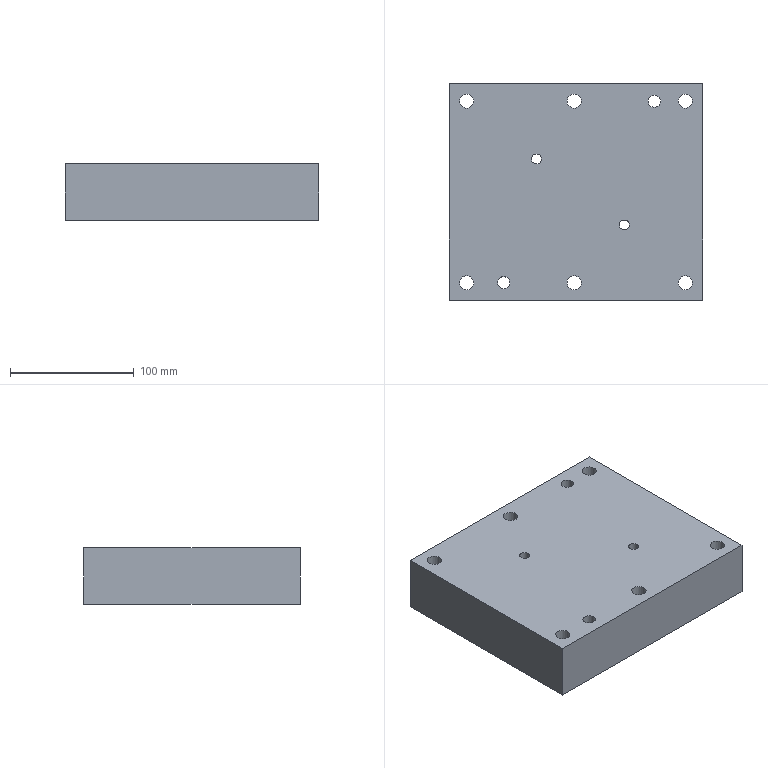Part | NX | features solid 2 | 1 solid | 50 faces | box 205 x 175 x 46 mm | volume 1591427 mm3 | cylinder 24 | plane 14 | cone 12 | commonest cylinder face diameters 6.8 x6 11.507 x6 18.008 x6 8 x2 10 x2 12.505 x2
STEP:
#1=CARTESIAN_POINT('',(-87.57,-13.004,130.));
#2=VERTEX_POINT('',#1);
#3=CARTESIAN_POINT('',(-90.97,-13.004,130.));
#4=DIRECTION('',(0.,0.,1.));
#5=DIRECTION('',(1.,0.,0.));
#6=AXIS2_PLACEMENT_3D('',#3,#4,#5);
#7=CIRCLE('',#6,3.4);
#8=EDGE_CURVE('',#2,#2,#7,.F.);
#9=ORIENTED_EDGE('',*,*,#8,.T.);
#10=EDGE_LOOP('',(#9));
#11=FACE_BOUND('',#10,.T.);
#12=CARTESIAN_POINT('',(-90.97,-13.004,132.043));
#13=VERTEX_POINT('',#12);
#14=VERTEX_LOOP('',#13);
#15=FACE_BOUND('',#14,.T.);
#16=CARTESIAN_POINT('',(-90.97,-13.004,130.));
#17=DIRECTION('',(0.,0.,-1.));
#18=DIRECTION('',(-1.,0.,0.));
#19=AXIS2_PLACEMENT_3D('',#16,#17,#18);
#20=CONICAL_SURFACE('',#19,3.4,1.03);
#21=ADVANCED_FACE('',(#11,#15),#20,.F.);
#22=CARTESIAN_POINT('',(-94.37,-13.004,105.599));
#23=VERTEX_POINT('',#22);
#24=CARTESIAN_POINT('',(-90.97,-13.004,105.599));
#25=DIRECTION('',(0.,0.,-1.));
#26=DIRECTION('',(-1.,0.,0.));
#27=AXIS2_PLACEMENT_3D('',#24,#25,#26);
#28=CIRCLE('',#27,3.4);
#29=EDGE_CURVE('',#23,#23,#28,.T.);
#30=ORIENTED_EDGE('',*,*,#29,.T.);
#31=EDGE_LOOP('',(#30));
#32=FACE_BOUND('',#31,.T.);
#33=ORIENTED_EDGE('',*,*,#8,.F.);
#34=EDGE_LOOP('',(#33));
#35=FACE_BOUND('',#34,.T.);
#36=CARTESIAN_POINT('',(-90.97,-13.004,105.));
#37=DIRECTION('',(0.,0.,1.));
#38=DIRECTION('',(1.,0.,0.));
#39=AXIS2_PLACEMENT_3D('',#36,#37,#38);
#40=CYLINDRICAL_SURFACE('',#39,3.4);
#41=ADVANCED_FACE('',(#32,#35),#40,.F.);
#42=CARTESIAN_POINT('',(-87.101,-13.004,105.13));
#43=VERTEX_POINT('',#42);
#44=CARTESIAN_POINT('',(-90.97,-13.004,105.13));
#45=DIRECTION('',(0.,0.,1.));
#46=DIRECTION('',(1.,0.,0.));
#47=AXIS2_PLACEMENT_3D('',#44,#45,#46);
#48=CIRCLE('',#47,3.869);
#49=EDGE_CURVE('',#43,#43,#48,.F.);
#50=ORIENTED_EDGE('',*,*,#49,.T.);
#51=EDGE_LOOP('',(#50));
#52=FACE_BOUND('',#51,.T.);
#53=ORIENTED_EDGE('',*,*,#29,.F.);
#54=EDGE_LOOP('',(#53));
#55=FACE_BOUND('',#54,.T.);
#56=CARTESIAN_POINT('',(-90.97,-13.004,105.599));
#57=DIRECTION('',(0.,0.,-1.));
#58=DIRECTION('',(-1.,0.,0.));
#59=AXIS2_PLACEMENT_3D('',#56,#57,#58);
#60=CONICAL_SURFACE('',#59,3.4,0.7854);
#61=ADVANCED_FACE('',(#52,#55),#60,.F.);
#62=CARTESIAN_POINT('',(-252.523,47.776,105.13));
#63=VERTEX_POINT('',#62);
#64=CARTESIAN_POINT('',(-47.523,47.776,105.13));
#65=VERTEX_POINT('',#64);
#66=CARTESIAN_POINT('',(-150.023,47.776,105.13));
#67=DIRECTION('',(1.,0.,0.));
#68=VECTOR('',#67,1000.);
#69=LINE('',#66,#68);
#70=EDGE_CURVE('',#63,#65,#69,.T.);
#71=ORIENTED_EDGE('',*,*,#70,.T.);
#72=CARTESIAN_POINT('',(-47.523,-127.224,105.13));
#73=VERTEX_POINT('',#72);
#74=CARTESIAN_POINT('',(-47.523,-39.724,105.13));
#75=DIRECTION('',(0.,-1.,0.));
#76=VECTOR('',#75,1000.);
#77=LINE('',#74,#76);
#78=EDGE_CURVE('',#73,#65,#77,.F.);
#79=ORIENTED_EDGE('',*,*,#78,.F.);
#80=CARTESIAN_POINT('',(-252.523,-127.224,105.13));
#81=VERTEX_POINT('',#80);
#82=CARTESIAN_POINT('',(-150.023,-127.224,105.13));
#83=DIRECTION('',(-1.,0.,0.));
#84=VECTOR('',#83,1000.);
#85=LINE('',#82,#84);
#86=EDGE_CURVE('',#81,#73,#85,.F.);
#87=ORIENTED_EDGE('',*,*,#86,.F.);
#88=CARTESIAN_POINT('',(-252.523,-39.724,105.13));
#89=DIRECTION('',(0.,1.,0.));
#90=VECTOR('',#89,1000.);
#91=LINE('',#88,#90);
#92=EDGE_CURVE('',#63,#81,#91,.F.);
#93=ORIENTED_EDGE('',*,*,#92,.F.);
#94=EDGE_LOOP('',(#71,#79,#87,#93));
#95=FACE_BOUND('',#94,.T.);
#96=CARTESIAN_POINT('',(-229.519,-113.224,105.13));
#97=VERTEX_POINT('',#96);
#98=CARTESIAN_POINT('',(-238.523,-113.224,105.13));
#99=DIRECTION('',(0.,0.,1.));
#100=DIRECTION('',(1.,0.,0.));
#101=AXIS2_PLACEMENT_3D('',#98,#99,#100);
#102=CIRCLE('',#101,9.004);
#103=EDGE_CURVE('',#97,#97,#102,.T.);
#104=ORIENTED_EDGE('',*,*,#103,.T.);
#105=EDGE_LOOP('',(#104));
#106=FACE_BOUND('',#105,.T.);
#107=CARTESIAN_POINT('',(-52.519,-113.224,105.13));
#108=VERTEX_POINT('',#107);
#109=CARTESIAN_POINT('',(-61.523,-113.224,105.13));
#110=DIRECTION('',(0.,0.,1.));
#111=DIRECTION('',(1.,0.,0.));
#112=AXIS2_PLACEMENT_3D('',#109,#110,#111);
#113=CIRCLE('',#112,9.004);
#114=EDGE_CURVE('',#108,#108,#113,.F.);
#115=ORIENTED_EDGE('',*,*,#114,.F.);
#116=EDGE_LOOP('',(#115));
#117=FACE_BOUND('',#116,.T.);
#118=CARTESIAN_POINT('',(-202.271,-113.224,105.13));
#119=VERTEX_POINT('',#118);
#120=CARTESIAN_POINT('',(-208.523,-113.224,105.13));
#121=DIRECTION('',(0.,0.,1.));
#122=DIRECTION('',(1.,0.,0.));
#123=AXIS2_PLACEMENT_3D('',#120,#121,#122);
#124=CIRCLE('',#123,6.253);
#125=EDGE_CURVE('',#119,#119,#124,.T.);
#126=ORIENTED_EDGE('',*,*,#125,.T.);
#127=EDGE_LOOP('',(#126));
#128=FACE_BOUND('',#127,.T.);
#129=CARTESIAN_POINT('',(-142.519,33.776,105.13));
#130=VERTEX_POINT('',#129);
#131=CARTESIAN_POINT('',(-151.523,33.776,105.13));
#132=DIRECTION('',(0.,0.,1.));
#133=DIRECTION('',(1.,0.,0.));
#134=AXIS2_PLACEMENT_3D('',#131,#132,#133);
#135=CIRCLE('',#134,9.004);
#136=EDGE_CURVE('',#130,#130,#135,.F.);
#137=ORIENTED_EDGE('',*,*,#136,.F.);
#138=EDGE_LOOP('',(#137));
#139=FACE_BOUND('',#138,.T.);
#140=ORIENTED_EDGE('',*,*,#49,.F.);
#141=EDGE_LOOP('',(#140));
#142=FACE_BOUND('',#141,.T.);
#143=CARTESIAN_POINT('',(-146.154,-13.004,105.13));
#144=VERTEX_POINT('',#143);
#145=CARTESIAN_POINT('',(-150.023,-13.004,105.13));
#146=DIRECTION('',(0.,0.,1.));
#147=DIRECTION('',(1.,0.,0.));
#148=AXIS2_PLACEMENT_3D('',#145,#146,#147);
#149=CIRCLE('',#148,3.869);
#150=EDGE_CURVE('',#144,#144,#149,.F.);
#151=ORIENTED_EDGE('',*,*,#150,.F.);
#152=EDGE_LOOP('',(#151));
#153=FACE_BOUND('',#152,.T.);
#154=CARTESIAN_POINT('',(-203.207,-13.004,105.13));
#155=VERTEX_POINT('',#154);
#156=CARTESIAN_POINT('',(-207.076,-13.004,105.13));
#157=DIRECTION('',(0.,0.,1.));
#158=DIRECTION('',(1.,0.,0.));
#159=AXIS2_PLACEMENT_3D('',#156,#157,#158);
#160=CIRCLE('',#159,3.869);
#161=EDGE_CURVE('',#155,#155,#160,.T.);
#162=ORIENTED_EDGE('',*,*,#161,.T.);
#163=EDGE_LOOP('',(#162));
#164=FACE_BOUND('',#163,.T.);
#165=CARTESIAN_POINT('',(-203.207,-66.444,105.13));
#166=VERTEX_POINT('',#165);
#167=CARTESIAN_POINT('',(-207.076,-66.444,105.13));
#168=DIRECTION('',(0.,0.,1.));
#169=DIRECTION('',(1.,0.,0.));
#170=AXIS2_PLACEMENT_3D('',#167,#168,#169);
#171=CIRCLE('',#170,3.869);
#172=EDGE_CURVE('',#166,#166,#171,.T.);
#173=ORIENTED_EDGE('',*,*,#172,.T.);
#174=EDGE_LOOP('',(#173));
#175=FACE_BOUND('',#174,.T.);
#176=CARTESIAN_POINT('',(-146.154,-66.444,105.13));
#177=VERTEX_POINT('',#176);
#178=CARTESIAN_POINT('',(-150.023,-66.444,105.13));
#179=DIRECTION('',(0.,0.,1.));
#180=DIRECTION('',(1.,0.,0.));
#181=AXIS2_PLACEMENT_3D('',#178,#179,#180);
#182=CIRCLE('',#181,3.869);
#183=EDGE_CURVE('',#177,#177,#182,.F.);
#184=ORIENTED_EDGE('',*,*,#183,.F.);
#185=EDGE_LOOP('',(#184));
#186=FACE_BOUND('',#185,.T.);
#187=CARTESIAN_POINT('',(-87.101,-66.444,105.13));
#188=VERTEX_POINT('',#187);
#189=CARTESIAN_POINT('',(-90.97,-66.444,105.13));
#190=DIRECTION('',(0.,0.,1.));
#191=DIRECTION('',(1.,0.,0.));
#192=AXIS2_PLACEMENT_3D('',#189,#190,#191);
#193=CIRCLE('',#192,3.869);
#194=EDGE_CURVE('',#188,#188,#193,.F.);
#195=ORIENTED_EDGE('',*,*,#194,.F.);
#196=EDGE_LOOP('',(#195));
#197=FACE_BOUND('',#196,.T.);
#198=CARTESIAN_POINT('',(-111.38,-62.465,105.13));
#199=VERTEX_POINT('',#198);
#200=CARTESIAN_POINT('',(-110.97,-66.444,105.13));
#201=DIRECTION('',(0.,0.,1.));
#202=DIRECTION('',(-0.1024,0.9947,0.));
#203=AXIS2_PLACEMENT_3D('',#200,#201,#202);
#204=ELLIPSE('',#203,4.,4.);
#205=EDGE_CURVE('',#199,#199,#204,.T.);
#206=ORIENTED_EDGE('',*,*,#205,.T.);
#207=EDGE_LOOP('',(#206));
#208=FACE_BOUND('',#207,.T.);
#209=CARTESIAN_POINT('',(-182.486,-9.025,105.13));
#210=VERTEX_POINT('',#209);
#211=CARTESIAN_POINT('',(-182.076,-13.004,105.13));
#212=DIRECTION('',(0.,0.,1.));
#213=DIRECTION('',(-0.1024,0.9947,0.));
#214=AXIS2_PLACEMENT_3D('',#211,#212,#213);
#215=ELLIPSE('',#214,4.,4.);
#216=EDGE_CURVE('',#210,#210,#215,.T.);
#217=ORIENTED_EDGE('',*,*,#216,.T.);
#218=EDGE_LOOP('',(#217));
#219=FACE_BOUND('',#218,.T.);
#220=CARTESIAN_POINT('',(-142.519,-113.224,105.13));
#221=VERTEX_POINT('',#220);
#222=CARTESIAN_POINT('',(-151.523,-113.224,105.13));
#223=DIRECTION('',(0.,0.,1.));
#224=DIRECTION('',(1.,0.,0.));
#225=AXIS2_PLACEMENT_3D('',#222,#223,#224);
#226=CIRCLE('',#225,9.004);
#227=EDGE_CURVE('',#221,#221,#226,.F.);
#228=ORIENTED_EDGE('',*,*,#227,.F.);
#229=EDGE_LOOP('',(#228));
#230=FACE_BOUND('',#229,.T.);
#231=CARTESIAN_POINT('',(-80.271,33.776,105.13));
#232=VERTEX_POINT('',#231);
#233=CARTESIAN_POINT('',(-86.523,33.776,105.13));
#234=DIRECTION('',(0.,0.,1.));
#235=DIRECTION('',(1.,0.,0.));
#236=AXIS2_PLACEMENT_3D('',#233,#234,#235);
#237=CIRCLE('',#236,6.253);
#238=EDGE_CURVE('',#232,#232,#237,.T.);
#239=ORIENTED_EDGE('',*,*,#238,.T.);
#240=EDGE_LOOP('',(#239));
#241=FACE_BOUND('',#240,.T.);
#242=CARTESIAN_POINT('',(-229.519,33.776,105.13));
#243=VERTEX_POINT('',#242);
#244=CARTESIAN_POINT('',(-238.523,33.776,105.13));
#245=DIRECTION('',(0.,0.,1.));
#246=DIRECTION('',(1.,0.,0.));
#247=AXIS2_PLACEMENT_3D('',#244,#245,#246);
#248=CIRCLE('',#247,9.004);
#249=EDGE_CURVE('',#243,#243,#248,.T.);
#250=ORIENTED_EDGE('',*,*,#249,.T.);
#251=EDGE_LOOP('',(#250));
#252=FACE_BOUND('',#251,.T.);
#253=CARTESIAN_POINT('',(-52.519,33.776,105.13));
#254=VERTEX_POINT('',#253);
#255=CARTESIAN_POINT('',(-61.523,33.776,105.13));
#256=DIRECTION('',(0.,0.,1.));
#257=DIRECTION('',(1.,0.,0.));
#258=AXIS2_PLACEMENT_3D('',#255,#256,#257);
#259=CIRCLE('',#258,9.004);
#260=EDGE_CURVE('',#254,#254,#259,.F.);
#261=ORIENTED_EDGE('',*,*,#260,.F.);
#262=EDGE_LOOP('',(#261));
#263=FACE_BOUND('',#262,.T.);
#264=CARTESIAN_POINT('',(-150.023,-39.724,105.13));
#265=DIRECTION('',(0.,0.,1.));
#266=DIRECTION('',(1.,0.,0.));
#267=AXIS2_PLACEMENT_3D('',#264,#265,#266);
#268=PLANE('',#267);
#269=ADVANCED_FACE('',(#95,#106,#117,#128,#139,#142,#153,#164,#175,#186,#197,#208,#219,#230,#241,#252,#263),#268,.F.);
#270=CARTESIAN_POINT('',(-87.57,-66.444,129.999));
#271=VERTEX_POINT('',#270);
#272=CARTESIAN_POINT('',(-90.97,-66.444,129.999));
#273=DIRECTION('',(0.,0.,1.));
#274=DIRECTION('',(1.,0.,0.));
#275=AXIS2_PLACEMENT_3D('',#272,#273,#274);
#276=CIRCLE('',#275,3.4);
#277=EDGE_CURVE('',#271,#271,#276,.F.);
#278=ORIENTED_EDGE('',*,*,#277,.T.);
#279=EDGE_LOOP('',(#278));
#280=FACE_BOUND('',#279,.T.);
#281=CARTESIAN_POINT('',(-90.97,-66.444,132.042));
#282=VERTEX_POINT('',#281);
#283=VERTEX_LOOP('',#282);
#284=FACE_BOUND('',#283,.T.);
#285=CARTESIAN_POINT('',(-90.97,-66.444,129.999));
#286=DIRECTION('',(0.,0.,-1.));
#287=DIRECTION('',(-1.,0.,0.));
#288=AXIS2_PLACEMENT_3D('',#285,#286,#287);
#289=CONICAL_SURFACE('',#288,3.4,1.03);
#290=ADVANCED_FACE('',(#280,#284),#289,.F.);
#291=CARTESIAN_POINT('',(-94.37,-66.444,105.599));
#292=VERTEX_POINT('',#291);
#293=CARTESIAN_POINT('',(-90.97,-66.444,105.599));
#294=DIRECTION('',(0.,0.,-1.));
#295=DIRECTION('',(-1.,0.,0.));
#296=AXIS2_PLACEMENT_3D('',#293,#294,#295);
#297=CIRCLE('',#296,3.4);
#298=EDGE_CURVE('',#292,#292,#297,.T.);
#299=ORIENTED_EDGE('',*,*,#298,.T.);
#300=EDGE_LOOP('',(#299));
#301=FACE_BOUND('',#300,.T.);
#302=ORIENTED_EDGE('',*,*,#277,.F.);
#303=EDGE_LOOP('',(#302));
#304=FACE_BOUND('',#303,.T.);
#305=CARTESIAN_POINT('',(-90.97,-66.444,104.999));
#306=DIRECTION('',(0.,0.,1.));
#307=DIRECTION('',(1.,0.,0.));
#308=AXIS2_PLACEMENT_3D('',#305,#306,#307);
#309=CYLINDRICAL_SURFACE('',#308,3.4);
#310=ADVANCED_FACE('',(#301,#304),#309,.F.);
#311=ORIENTED_EDGE('',*,*,#194,.T.);
#312=EDGE_LOOP('',(#311));
#313=FACE_BOUND('',#312,.T.);
#314=ORIENTED_EDGE('',*,*,#298,.F.);
#315=EDGE_LOOP('',(#314));
#316=FACE_BOUND('',#315,.T.);
#317=CARTESIAN_POINT('',(-90.97,-66.444,105.599));
#318=DIRECTION('',(0.,0.,-1.));
#319=DIRECTION('',(-1.,0.,0.));
#320=AXIS2_PLACEMENT_3D('',#317,#318,#319);
#321=CONICAL_SURFACE('',#320,3.4,0.7854);
#322=ADVANCED_FACE('',(#313,#316),#321,.F.);
#323=CARTESIAN_POINT('',(-146.623,-66.444,130.));
#324=VERTEX_POINT('',#323);
#325=CARTESIAN_POINT('',(-150.023,-66.444,130.));
#326=DIRECTION('',(0.,0.,1.));
#327=DIRECTION('',(1.,0.,0.));
#328=AXIS2_PLACEMENT_3D('',#325,#326,#327);
#329=CIRCLE('',#328,3.4);
#330=EDGE_CURVE('',#324,#324,#329,.F.);
#331=ORIENTED_EDGE('',*,*,#330,.T.);
#332=EDGE_LOOP('',(#331));
#333=FACE_BOUND('',#332,.T.);
#334=CARTESIAN_POINT('',(-150.023,-66.444,132.042));
#335=VERTEX_POINT('',#334);
#336=VERTEX_LOOP('',#335);
#337=FACE_BOUND('',#336,.T.);
#338=CARTESIAN_POINT('',(-150.023,-66.444,130.));
#339=DIRECTION('',(0.,0.,-1.));
#340=DIRECTION('',(-1.,0.,0.));
#341=AXIS2_PLACEMENT_3D('',#338,#339,#340);
#342=CONICAL_SURFACE('',#341,3.4,1.03);
#343=ADVANCED_FACE('',(#333,#337),#342,.F.);
#344=CARTESIAN_POINT('',(-153.423,-66.444,105.599));
#345=VERTEX_POINT('',#344);
#346=CARTESIAN_POINT('',(-150.023,-66.444,105.599));
#347=DIRECTION('',(0.,0.,-1.));
#348=DIRECTION('',(-1.,0.,0.));
#349=AXIS2_PLACEMENT_3D('',#346,#347,#348);
#350=CIRCLE('',#349,3.4);
#351=EDGE_CURVE('',#345,#345,#350,.T.);
#352=ORIENTED_EDGE('',*,*,#351,.T.);
#353=EDGE_LOOP('',(#352));
#354=FACE_BOUND('',#353,.T.);
#355=ORIENTED_EDGE('',*,*,#330,.F.);
#356=EDGE_LOOP('',(#355));
#357=FACE_BOUND('',#356,.T.);
#358=CARTESIAN_POINT('',(-150.023,-66.444,105.));
#359=DIRECTION('',(0.,0.,1.));
#360=DIRECTION('',(1.,0.,0.));
#361=AXIS2_PLACEMENT_3D('',#358,#359,#360);
#362=CYLINDRICAL_SURFACE('',#361,3.4);
#363=ADVANCED_FACE('',(#354,#357),#362,.F.);
#364=ORIENTED_EDGE('',*,*,#183,.T.);
#365=EDGE_LOOP('',(#364));
#366=FACE_BOUND('',#365,.T.);
#367=ORIENTED_EDGE('',*,*,#351,.F.);
#368=EDGE_LOOP('',(#367));
#369=FACE_BOUND('',#368,.T.);
#370=CARTESIAN_POINT('',(-150.023,-66.444,105.599));
#371=DIRECTION('',(0.,0.,-1.));
#372=DIRECTION('',(-1.,0.,0.));
#373=AXIS2_PLACEMENT_3D('',#370,#371,#372);
#374=CONICAL_SURFACE('',#373,3.4,0.7854);
#375=ADVANCED_FACE('',(#366,#369),#374,.F.);
#376=CARTESIAN_POINT('',(-203.676,-66.444,130.));
#377=VERTEX_POINT('',#376);
#378=CARTESIAN_POINT('',(-207.076,-66.444,130.));
#379=DIRECTION('',(0.,0.,1.));
#380=DIRECTION('',(1.,0.,0.));
#381=AXIS2_PLACEMENT_3D('',#378,#379,#380);
#382=CIRCLE('',#381,3.4);
#383=EDGE_CURVE('',#377,#377,#382,.F.);
#384=ORIENTED_EDGE('',*,*,#383,.T.);
#385=EDGE_LOOP('',(#384));
#386=FACE_BOUND('',#385,.T.);
#387=CARTESIAN_POINT('',(-207.076,-66.444,132.043));
#388=VERTEX_POINT('',#387);
#389=VERTEX_LOOP('',#388);
#390=FACE_BOUND('',#389,.T.);
#391=CARTESIAN_POINT('',(-207.076,-66.444,130.));
#392=DIRECTION('',(0.,0.,-1.));
#393=DIRECTION('',(-1.,0.,0.));
#394=AXIS2_PLACEMENT_3D('',#391,#392,#393);
#395=CONICAL_SURFACE('',#394,3.4,1.03);
#396=ADVANCED_FACE('',(#386,#390),#395,.F.);
#397=CARTESIAN_POINT('',(-210.476,-66.444,105.599));
#398=VERTEX_POINT('',#397);
#399=CARTESIAN_POINT('',(-207.076,-66.444,105.599));
#400=DIRECTION('',(0.,0.,-1.));
#401=DIRECTION('',(-1.,0.,0.));
#402=AXIS2_PLACEMENT_3D('',#399,#400,#401);
#403=CIRCLE('',#402,3.4);
#404=EDGE_CURVE('',#398,#398,#403,.T.);
#405=ORIENTED_EDGE('',*,*,#404,.T.);
#406=EDGE_LOOP('',(#405));
#407=FACE_BOUND('',#406,.T.);
#408=ORIENTED_EDGE('',*,*,#383,.F.);
#409=EDGE_LOOP('',(#408));
#410=FACE_BOUND('',#409,.T.);
#411=CARTESIAN_POINT('',(-207.076,-66.444,105.));
#412=DIRECTION('',(0.,0.,1.));
#413=DIRECTION('',(1.,0.,0.));
#414=AXIS2_PLACEMENT_3D('',#411,#412,#413);
#415=CYLINDRICAL_SURFACE('',#414,3.4);
#416=ADVANCED_FACE('',(#407,#410),#415,.F.);
#417=ORIENTED_EDGE('',*,*,#172,.F.);
#418=EDGE_LOOP('',(#417));
#419=FACE_BOUND('',#418,.T.);
#420=ORIENTED_EDGE('',*,*,#404,.F.);
#421=EDGE_LOOP('',(#420));
#422=FACE_BOUND('',#421,.T.);
#423=CARTESIAN_POINT('',(-207.076,-66.444,105.599));
#424=DIRECTION('',(0.,0.,-1.));
#425=DIRECTION('',(-1.,0.,0.));
#426=AXIS2_PLACEMENT_3D('',#423,#424,#425);
#427=CONICAL_SURFACE('',#426,3.4,0.7854);
#428=ADVANCED_FACE('',(#419,#422),#427,.F.);
#429=CARTESIAN_POINT('',(-203.676,-13.004,130.));
#430=VERTEX_POINT('',#429);
#431=CARTESIAN_POINT('',(-207.076,-13.004,130.));
#432=DIRECTION('',(0.,0.,1.));
#433=DIRECTION('',(1.,0.,0.));
#434=AXIS2_PLACEMENT_3D('',#431,#432,#433);
#435=CIRCLE('',#434,3.4);
#436=EDGE_CURVE('',#430,#430,#435,.F.);
#437=ORIENTED_EDGE('',*,*,#436,.T.);
#438=EDGE_LOOP('',(#437));
#439=FACE_BOUND('',#438,.T.);
#440=CARTESIAN_POINT('',(-207.076,-13.004,132.043));
#441=VERTEX_POINT('',#440);
#442=VERTEX_LOOP('',#441);
#443=FACE_BOUND('',#442,.T.);
#444=CARTESIAN_POINT('',(-207.076,-13.004,130.));
#445=DIRECTION('',(0.,0.,-1.));
#446=DIRECTION('',(-1.,0.,0.));
#447=AXIS2_PLACEMENT_3D('',#444,#445,#446);
#448=CONICAL_SURFACE('',#447,3.4,1.03);
#449=ADVANCED_FACE('',(#439,#443),#448,.F.);
#450=CARTESIAN_POINT('',(-210.476,-13.004,105.599));
#451=VERTEX_POINT('',#450);
#452=CARTESIAN_POINT('',(-207.076,-13.004,105.599));
#453=DIRECTION('',(0.,0.,-1.));
#454=DIRECTION('',(-1.,0.,0.));
#455=AXIS2_PLACEMENT_3D('',#452,#453,#454);
#456=CIRCLE('',#455,3.4);
#457=EDGE_CURVE('',#451,#451,#456,.T.);
#458=ORIENTED_EDGE('',*,*,#457,.T.);
#459=EDGE_LOOP('',(#458));
#460=FACE_BOUND('',#459,.T.);
#461=ORIENTED_EDGE('',*,*,#436,.F.);
#462=EDGE_LOOP('',(#461));
#463=FACE_BOUND('',#462,.T.);
#464=CARTESIAN_POINT('',(-207.076,-13.004,105.));
#465=DIRECTION('',(0.,0.,1.));
#466=DIRECTION('',(1.,0.,0.));
#467=AXIS2_PLACEMENT_3D('',#464,#465,#466);
#468=CYLINDRICAL_SURFACE('',#467,3.4);
#469=ADVANCED_FACE('',(#460,#463),#468,.F.);
#470=ORIENTED_EDGE('',*,*,#161,.F.);
#471=EDGE_LOOP('',(#470));
#472=FACE_BOUND('',#471,.T.);
#473=ORIENTED_EDGE('',*,*,#457,.F.);
#474=EDGE_LOOP('',(#473));
#475=FACE_BOUND('',#474,.T.);
#476=CARTESIAN_POINT('',(-207.076,-13.004,105.599));
#477=DIRECTION('',(0.,0.,-1.));
#478=DIRECTION('',(-1.,0.,0.));
#479=AXIS2_PLACEMENT_3D('',#476,#477,#478);
#480=CONICAL_SURFACE('',#479,3.4,0.7854);
#481=ADVANCED_FACE('',(#472,#475),#480,.F.);
#482=CARTESIAN_POINT('',(-146.623,-13.004,130.));
#483=VERTEX_POINT('',#482);
#484=CARTESIAN_POINT('',(-150.023,-13.004,130.));
#485=DIRECTION('',(0.,0.,1.));
#486=DIRECTION('',(1.,0.,0.));
#487=AXIS2_PLACEMENT_3D('',#484,#485,#486);
#488=CIRCLE('',#487,3.4);
#489=EDGE_CURVE('',#483,#483,#488,.F.);
#490=ORIENTED_EDGE('',*,*,#489,.T.);
#491=EDGE_LOOP('',(#490));
#492=FACE_BOUND('',#491,.T.);
#493=CARTESIAN_POINT('',(-150.023,-13.004,132.043));
#494=VERTEX_POINT('',#493);
#495=VERTEX_LOOP('',#494);
#496=FACE_BOUND('',#495,.T.);
#497=CARTESIAN_POINT('',(-150.023,-13.004,130.));
#498=DIRECTION('',(0.,0.,-1.));
#499=DIRECTION('',(-1.,0.,0.));
#500=AXIS2_PLACEMENT_3D('',#497,#498,#499);
#501=CONICAL_SURFACE('',#500,3.4,1.03);
#502=ADVANCED_FACE('',(#492,#496),#501,.F.);
#503=CARTESIAN_POINT('',(-153.423,-13.004,105.599));
#504=VERTEX_POINT('',#503);
#505=CARTESIAN_POINT('',(-150.023,-13.004,105.599));
#506=DIRECTION('',(0.,0.,-1.));
#507=DIRECTION('',(-1.,0.,0.));
#508=AXIS2_PLACEMENT_3D('',#505,#506,#507);
#509=CIRCLE('',#508,3.4);
#510=EDGE_CURVE('',#504,#504,#509,.T.);
#511=ORIENTED_EDGE('',*,*,#510,.T.);
#512=EDGE_LOOP('',(#511));
#513=FACE_BOUND('',#512,.T.);
#514=ORIENTED_EDGE('',*,*,#489,.F.);
#515=EDGE_LOOP('',(#514));
#516=FACE_BOUND('',#515,.T.);
#517=CARTESIAN_POINT('',(-150.023,-13.004,105.));
#518=DIRECTION('',(0.,0.,1.));
#519=DIRECTION('',(1.,0.,0.));
#520=AXIS2_PLACEMENT_3D('',#517,#518,#519);
#521=CYLINDRICAL_SURFACE('',#520,3.4);
#522=ADVANCED_FACE('',(#513,#516),#521,.F.);
#523=ORIENTED_EDGE('',*,*,#150,.T.);
#524=EDGE_LOOP('',(#523));
#525=FACE_BOUND('',#524,.T.);
#526=ORIENTED_EDGE('',*,*,#510,.F.);
#527=EDGE_LOOP('',(#526));
#528=FACE_BOUND('',#527,.T.);
#529=CARTESIAN_POINT('',(-150.023,-13.004,105.599));
#530=DIRECTION('',(0.,0.,-1.));
#531=DIRECTION('',(-1.,0.,0.));
#532=AXIS2_PLACEMENT_3D('',#529,#530,#531);
#533=CONICAL_SURFACE('',#532,3.4,0.7854);
#534=ADVANCED_FACE('',(#525,#528),#533,.F.);
#535=CARTESIAN_POINT('',(-67.277,33.776,117.999));
#536=VERTEX_POINT('',#535);
#537=CARTESIAN_POINT('',(-61.523,33.776,117.999));
#538=DIRECTION('',(0.,0.,1.));
#539=DIRECTION('',(-1.,0.,0.));
#540=AXIS2_PLACEMENT_3D('',#537,#538,#539);
#541=CIRCLE('',#540,5.753);
#542=EDGE_CURVE('',#536,#536,#541,.T.);
#543=ORIENTED_EDGE('',*,*,#542,.T.);
#544=EDGE_LOOP('',(#543));
#545=FACE_BOUND('',#544,.T.);
#546=CARTESIAN_POINT('',(-70.527,33.776,117.999));
#547=VERTEX_POINT('',#546);
#548=CARTESIAN_POINT('',(-61.523,33.776,117.999));
#549=DIRECTION('',(0.,0.,-1.));
#550=DIRECTION('',(-1.,0.,0.));
#551=AXIS2_PLACEMENT_3D('',#548,#549,#550);
#552=CIRCLE('',#551,9.004);
#553=EDGE_CURVE('',#547,#547,#552,.F.);
#554=ORIENTED_EDGE('',*,*,#553,.F.);
#555=EDGE_LOOP('',(#554));
#556=FACE_BOUND('',#555,.T.);
#557=CARTESIAN_POINT('',(-61.523,33.776,117.999));
#558=DIRECTION('',(0.,0.,1.));
#559=DIRECTION('',(-1.,0.,0.));
#560=AXIS2_PLACEMENT_3D('',#557,#558,#559);
#561=PLANE('',#560);
#562=ADVANCED_FACE('',(#545,#556),#561,.F.);
#563=ORIENTED_EDGE('',*,*,#260,.T.);
#564=EDGE_LOOP('',(#563));
#565=FACE_BOUND('',#564,.T.);
#566=ORIENTED_EDGE('',*,*,#553,.T.);
#567=EDGE_LOOP('',(#566));
#568=FACE_BOUND('',#567,.T.);
#569=CARTESIAN_POINT('',(-61.523,33.776,104.999));
#570=DIRECTION('',(0.,0.,1.));
#571=DIRECTION('',(-1.,0.,0.));
#572=AXIS2_PLACEMENT_3D('',#569,#570,#571);
#573=CYLINDRICAL_SURFACE('',#572,9.004);
#574=ADVANCED_FACE('',(#565,#568),#573,.F.);
#575=CARTESIAN_POINT('',(-67.277,33.776,151.13));
#576=VERTEX_POINT('',#575);
#577=CARTESIAN_POINT('',(-61.523,33.776,151.13));
#578=DIRECTION('',(0.,0.,-1.));
#579=DIRECTION('',(-1.,0.,0.));
#580=AXIS2_PLACEMENT_3D('',#577,#578,#579);
#581=CIRCLE('',#580,5.753);
#582=EDGE_CURVE('',#576,#576,#581,.F.);
#583=ORIENTED_EDGE('',*,*,#582,.T.);
#584=EDGE_LOOP('',(#583));
#585=FACE_BOUND('',#584,.T.);
#586=ORIENTED_EDGE('',*,*,#542,.F.);
#587=EDGE_LOOP('',(#586));
#588=FACE_BOUND('',#587,.T.);
#589=CARTESIAN_POINT('',(-61.523,33.776,101.999));
#590=DIRECTION('',(0.,0.,1.));
#591=DIRECTION('',(-1.,0.,0.));
#592=AXIS2_PLACEMENT_3D('',#589,#590,#591);
#593=CYLINDRICAL_SURFACE('',#592,5.753);
#594=ADVANCED_FACE('',(#585,#588),#593,.F.);
#595=CARTESIAN_POINT('',(-244.277,-113.224,117.999));
#596=VERTEX_POINT('',#595);
#597=CARTESIAN_POINT('',(-238.523,-113.224,117.999));
#598=DIRECTION('',(0.,0.,1.));
#599=DIRECTION('',(-1.,0.,0.));
#600=AXIS2_PLACEMENT_3D('',#597,#598,#599);
#601=CIRCLE('',#600,5.753);
#602=EDGE_CURVE('',#596,#596,#601,.T.);
#603=ORIENTED_EDGE('',*,*,#602,.T.);
#604=EDGE_LOOP('',(#603));
#605=FACE_BOUND('',#604,.T.);
#606=CARTESIAN_POINT('',(-247.527,-113.224,117.999));
#607=VERTEX_POINT('',#606);
#608=CARTESIAN_POINT('',(-238.523,-113.224,117.999));
#609=DIRECTION('',(0.,0.,-1.));
#610=DIRECTION('',(-1.,0.,0.));
#611=AXIS2_PLACEMENT_3D('',#608,#609,#610);
#612=CIRCLE('',#611,9.004);
#613=EDGE_CURVE('',#607,#607,#612,.F.);
#614=ORIENTED_EDGE('',*,*,#613,.F.);
#615=EDGE_LOOP('',(#614));
#616=FACE_BOUND('',#615,.T.);
#617=CARTESIAN_POINT('',(-238.523,-113.224,117.999));
#618=DIRECTION('',(0.,0.,1.));
#619=DIRECTION('',(-1.,0.,0.));
#620=AXIS2_PLACEMENT_3D('',#617,#618,#619);
#621=PLANE('',#620);
#622=ADVANCED_FACE('',(#605,#616),#621,.F.);
#623=ORIENTED_EDGE('',*,*,#103,.F.);
#624=EDGE_LOOP('',(#623));
#625=FACE_BOUND('',#624,.T.);
#626=ORIENTED_EDGE('',*,*,#613,.T.);
#627=EDGE_LOOP('',(#626));
#628=FACE_BOUND('',#627,.T.);
#629=CARTESIAN_POINT('',(-238.523,-113.224,104.999));
#630=DIRECTION('',(0.,0.,1.));
#631=DIRECTION('',(-1.,0.,0.));
#632=AXIS2_PLACEMENT_3D('',#629,#630,#631);
#633=CYLINDRICAL_SURFACE('',#632,9.004);
#634=ADVANCED_FACE('',(#625,#628),#633,.F.);
#635=CARTESIAN_POINT('',(-244.277,-113.224,151.13));
#636=VERTEX_POINT('',#635);
#637=CARTESIAN_POINT('',(-238.523,-113.224,151.13));
#638=DIRECTION('',(0.,0.,-1.));
#639=DIRECTION('',(-1.,0.,0.));
#640=AXIS2_PLACEMENT_3D('',#637,#638,#639);
#641=CIRCLE('',#640,5.753);
#642=EDGE_CURVE('',#636,#636,#641,.F.);
#643=ORIENTED_EDGE('',*,*,#642,.T.);
#644=EDGE_LOOP('',(#643));
#645=FACE_BOUND('',#644,.T.);
#646=ORIENTED_EDGE('',*,*,#602,.F.);
#647=EDGE_LOOP('',(#646));
#648=FACE_BOUND('',#647,.T.);
#649=CARTESIAN_POINT('',(-238.523,-113.224,101.999));
#650=DIRECTION('',(0.,0.,1.));
#651=DIRECTION('',(-1.,0.,0.));
#652=AXIS2_PLACEMENT_3D('',#649,#650,#651);
#653=CYLINDRICAL_SURFACE('',#652,5.753);
#654=ADVANCED_FACE('',(#645,#648),#653,.F.);
#655=CARTESIAN_POINT('',(-244.277,33.776,117.999));
#656=VERTEX_POINT('',#655);
#657=CARTESIAN_POINT('',(-238.523,33.776,117.999));
#658=DIRECTION('',(0.,0.,1.));
#659=DIRECTION('',(-1.,0.,0.));
#660=AXIS2_PLACEMENT_3D('',#657,#658,#659);
#661=CIRCLE('',#660,5.753);
#662=EDGE_CURVE('',#656,#656,#661,.T.);
#663=ORIENTED_EDGE('',*,*,#662,.T.);
#664=EDGE_LOOP('',(#663));
#665=FACE_BOUND('',#664,.T.);
#666=CARTESIAN_POINT('',(-247.527,33.776,117.999));
#667=VERTEX_POINT('',#666);
#668=CARTESIAN_POINT('',(-238.523,33.776,117.999));
#669=DIRECTION('',(0.,0.,-1.));
#670=DIRECTION('',(-1.,0.,0.));
#671=AXIS2_PLACEMENT_3D('',#668,#669,#670);
#672=CIRCLE('',#671,9.004);
#673=EDGE_CURVE('',#667,#667,#672,.F.);
#674=ORIENTED_EDGE('',*,*,#673,.F.);
#675=EDGE_LOOP('',(#674));
#676=FACE_BOUND('',#675,.T.);
#677=CARTESIAN_POINT('',(-238.523,33.776,117.999));
#678=DIRECTION('',(0.,0.,1.));
#679=DIRECTION('',(-1.,0.,0.));
#680=AXIS2_PLACEMENT_3D('',#677,#678,#679);
#681=PLANE('',#680);
#682=ADVANCED_FACE('',(#665,#676),#681,.F.);
#683=ORIENTED_EDGE('',*,*,#249,.F.);
#684=EDGE_LOOP('',(#683));
#685=FACE_BOUND('',#684,.T.);
#686=ORIENTED_EDGE('',*,*,#673,.T.);
#687=EDGE_LOOP('',(#686));
#688=FACE_BOUND('',#687,.T.);
#689=CARTESIAN_POINT('',(-238.523,33.776,104.999));
#690=DIRECTION('',(0.,0.,1.));
#691=DIRECTION('',(-1.,0.,0.));
#692=AXIS2_PLACEMENT_3D('',#689,#690,#691);
#693=CYLINDRICAL_SURFACE('',#692,9.004);
#694=ADVANCED_FACE('',(#685,#688),#693,.F.);
#695=CARTESIAN_POINT('',(-244.277,33.776,151.13));
#696=VERTEX_POINT('',#695);
#697=CARTESIAN_POINT('',(-238.523,33.776,151.13));
#698=DIRECTION('',(0.,0.,-1.));
#699=DIRECTION('',(-1.,0.,0.));
#700=AXIS2_PLACEMENT_3D('',#697,#698,#699);
#701=CIRCLE('',#700,5.753);
#702=EDGE_CURVE('',#696,#696,#701,.F.);
#703=ORIENTED_EDGE('',*,*,#702,.T.);
#704=EDGE_LOOP('',(#703));
#705=FACE_BOUND('',#704,.T.);
#706=ORIENTED_EDGE('',*,*,#662,.F.);
#707=EDGE_LOOP('',(#706));
#708=FACE_BOUND('',#707,.T.);
#709=CARTESIAN_POINT('',(-238.523,33.776,101.999));
#710=DIRECTION('',(0.,0.,1.));
#711=DIRECTION('',(-1.,0.,0.));
#712=AXIS2_PLACEMENT_3D('',#709,#710,#711);
#713=CYLINDRICAL_SURFACE('',#712,5.753);
#714=ADVANCED_FACE('',(#705,#708),#713,.F.);
#715=CARTESIAN_POINT('',(-67.277,-113.224,117.999));
#716=VERTEX_POINT('',#715);
#717=CARTESIAN_POINT('',(-61.523,-113.224,117.999));
#718=DIRECTION('',(0.,0.,1.));
#719=DIRECTION('',(-1.,0.,0.));
#720=AXIS2_PLACEMENT_3D('',#717,#718,#719);
#721=CIRCLE('',#720,5.753);
#722=EDGE_CURVE('',#716,#716,#721,.T.);
#723=ORIENTED_EDGE('',*,*,#722,.T.);
#724=EDGE_LOOP('',(#723));
#725=FACE_BOUND('',#724,.T.);
#726=CARTESIAN_POINT('',(-70.527,-113.224,117.999));
#727=VERTEX_POINT('',#726);
#728=CARTESIAN_POINT('',(-61.523,-113.224,117.999));
#729=DIRECTION('',(0.,0.,-1.));
#730=DIRECTION('',(-1.,0.,0.));
#731=AXIS2_PLACEMENT_3D('',#728,#729,#730);
#732=CIRCLE('',#731,9.004);
#733=EDGE_CURVE('',#727,#727,#732,.F.);
#734=ORIENTED_EDGE('',*,*,#733,.F.);
#735=EDGE_LOOP('',(#734));
#736=FACE_BOUND('',#735,.T.);
#737=CARTESIAN_POINT('',(-61.523,-113.224,117.999));
#738=DIRECTION('',(0.,0.,1.));
#739=DIRECTION('',(-1.,0.,0.));
#740=AXIS2_PLACEMENT_3D('',#737,#738,#739);
#741=PLANE('',#740);
#742=ADVANCED_FACE('',(#725,#736),#741,.F.);
#743=ORIENTED_EDGE('',*,*,#114,.T.);
#744=EDGE_LOOP('',(#743));
#745=FACE_BOUND('',#744,.T.);
#746=ORIENTED_EDGE('',*,*,#733,.T.);
#747=EDGE_LOOP('',(#746));
#748=FACE_BOUND('',#747,.T.);
#749=CARTESIAN_POINT('',(-61.523,-113.224,104.999));
#750=DIRECTION('',(0.,0.,1.));
#751=DIRECTION('',(-1.,0.,0.));
#752=AXIS2_PLACEMENT_3D('',#749,#750,#751);
#753=CYLINDRICAL_SURFACE('',#752,9.004);
#754=ADVANCED_FACE('',(#745,#748),#753,.F.);
#755=CARTESIAN_POINT('',(-67.277,-113.224,151.13));
#756=VERTEX_POINT('',#755);
#757=CARTESIAN_POINT('',(-61.523,-113.224,151.13));
#758=DIRECTION('',(0.,0.,-1.));
#759=DIRECTION('',(-1.,0.,0.));
#760=AXIS2_PLACEMENT_3D('',#757,#758,#759);
#761=CIRCLE('',#760,5.753);
#762=EDGE_CURVE('',#756,#756,#761,.F.);
#763=ORIENTED_EDGE('',*,*,#762,.T.);
#764=EDGE_LOOP('',(#763));
#765=FACE_BOUND('',#764,.T.);
#766=ORIENTED_EDGE('',*,*,#722,.F.);
#767=EDGE_LOOP('',(#766));
#768=FACE_BOUND('',#767,.T.);
#769=CARTESIAN_POINT('',(-61.523,-113.224,101.999));
#770=DIRECTION('',(0.,0.,1.));
#771=DIRECTION('',(-1.,0.,0.));
#772=AXIS2_PLACEMENT_3D('',#769,#770,#771);
#773=CYLINDRICAL_SURFACE('',#772,5.753);
#774=ADVANCED_FACE('',(#765,#768),#773,.F.);
#775=CARTESIAN_POINT('',(-91.523,33.776,116.999));
#776=VERTEX_POINT('',#775);
#777=CARTESIAN_POINT('',(-86.523,33.776,116.999));
#778=DIRECTION('',(0.,0.,1.));
#779=DIRECTION('',(-1.,0.,0.));
#780=AXIS2_PLACEMENT_3D('',#777,#778,#779);
#781=CIRCLE('',#780,5.);
#782=EDGE_CURVE('',#776,#776,#781,.T.);
#783=ORIENTED_EDGE('',*,*,#782,.T.);
#784=EDGE_LOOP('',(#783));
#785=FACE_BOUND('',#784,.T.);
#786=CARTESIAN_POINT('',(-92.776,33.776,116.999));
#787=VERTEX_POINT('',#786);
#788=CARTESIAN_POINT('',(-86.523,33.776,116.999));
#789=DIRECTION('',(0.,0.,-1.));
#790=DIRECTION('',(-1.,0.,0.));
#791=AXIS2_PLACEMENT_3D('',#788,#789,#790);
#792=CIRCLE('',#791,6.253);
#793=EDGE_CURVE('',#787,#787,#792,.F.);
#794=ORIENTED_EDGE('',*,*,#793,.F.);
#795=EDGE_LOOP('',(#794));
#796=FACE_BOUND('',#795,.T.);
#797=CARTESIAN_POINT('',(-86.523,33.776,116.999));
#798=DIRECTION('',(0.,0.,1.));
#799=DIRECTION('',(-1.,0.,0.));
#800=AXIS2_PLACEMENT_3D('',#797,#798,#799);
#801=PLANE('',#800);
#802=ADVANCED_FACE('',(#785,#796),#801,.F.);
#803=ORIENTED_EDGE('',*,*,#238,.F.);
#804=EDGE_LOOP('',(#803));
#805=FACE_BOUND('',#804,.T.);
#806=ORIENTED_EDGE('',*,*,#793,.T.);
#807=EDGE_LOOP('',(#806));
#808=FACE_BOUND('',#807,.T.);
#809=CARTESIAN_POINT('',(-86.523,33.776,101.999));
#810=DIRECTION('',(0.,0.,1.));
#811=DIRECTION('',(-1.,0.,0.));
#812=AXIS2_PLACEMENT_3D('',#809,#810,#811);
#813=CYLINDRICAL_SURFACE('',#812,6.253);
#814=ADVANCED_FACE('',(#805,#808),#813,.F.);
#815=CARTESIAN_POINT('',(-91.523,33.776,151.13));
#816=VERTEX_POINT('',#815);
#817=CARTESIAN_POINT('',(-86.523,33.776,151.13));
#818=DIRECTION('',(0.,0.,-1.));
#819=DIRECTION('',(-1.,0.,0.));
#820=AXIS2_PLACEMENT_3D('',#817,#818,#819);
#821=CIRCLE('',#820,5.);
#822=EDGE_CURVE('',#816,#816,#821,.F.);
#823=ORIENTED_EDGE('',*,*,#822,.T.);
#824=EDGE_LOOP('',(#823));
#825=FACE_BOUND('',#824,.T.);
#826=ORIENTED_EDGE('',*,*,#782,.F.);
#827=EDGE_LOOP('',(#826));
#828=FACE_BOUND('',#827,.T.);
#829=CARTESIAN_POINT('',(-86.523,33.776,101.999));
#830=DIRECTION('',(0.,0.,1.));
#831=DIRECTION('',(-1.,0.,0.));
#832=AXIS2_PLACEMENT_3D('',#829,#830,#831);
#833=CYLINDRICAL_SURFACE('',#832,5.);
#834=ADVANCED_FACE('',(#825,#828),#833,.F.);
#835=CARTESIAN_POINT('',(-213.523,-113.224,116.999));
#836=VERTEX_POINT('',#835);
#837=CARTESIAN_POINT('',(-208.523,-113.224,116.999));
#838=DIRECTION('',(0.,0.,1.));
#839=DIRECTION('',(-1.,0.,0.));
#840=AXIS2_PLACEMENT_3D('',#837,#838,#839);
#841=CIRCLE('',#840,5.);
#842=EDGE_CURVE('',#836,#836,#841,.T.);
#843=ORIENTED_EDGE('',*,*,#842,.T.);
#844=EDGE_LOOP('',(#843));
#845=FACE_BOUND('',#844,.T.);
#846=CARTESIAN_POINT('',(-214.776,-113.224,116.999));
#847=VERTEX_POINT('',#846);
#848=CARTESIAN_POINT('',(-208.523,-113.224,116.999));
#849=DIRECTION('',(0.,0.,-1.));
#850=DIRECTION('',(-1.,0.,0.));
#851=AXIS2_PLACEMENT_3D('',#848,#849,#850);
#852=CIRCLE('',#851,6.253);
#853=EDGE_CURVE('',#847,#847,#852,.F.);
#854=ORIENTED_EDGE('',*,*,#853,.F.);
#855=EDGE_LOOP('',(#854));
#856=FACE_BOUND('',#855,.T.);
#857=CARTESIAN_POINT('',(-208.523,-113.224,116.999));
#858=DIRECTION('',(0.,0.,1.));
#859=DIRECTION('',(-1.,0.,0.));
#860=AXIS2_PLACEMENT_3D('',#857,#858,#859);
#861=PLANE('',#860);
#862=ADVANCED_FACE('',(#845,#856),#861,.F.);
#863=ORIENTED_EDGE('',*,*,#125,.F.);
#864=EDGE_LOOP('',(#863));
#865=FACE_BOUND('',#864,.T.);
#866=ORIENTED_EDGE('',*,*,#853,.T.);
#867=EDGE_LOOP('',(#866));
#868=FACE_BOUND('',#867,.T.);
#869=CARTESIAN_POINT('',(-208.523,-113.224,101.999));
#870=DIRECTION('',(0.,0.,1.));
#871=DIRECTION('',(-1.,0.,0.));
#872=AXIS2_PLACEMENT_3D('',#869,#870,#871);
#873=CYLINDRICAL_SURFACE('',#872,6.253);
#874=ADVANCED_FACE('',(#865,#868),#873,.F.);
#875=CARTESIAN_POINT('',(-213.523,-113.224,151.13));
#876=VERTEX_POINT('',#875);
#877=CARTESIAN_POINT('',(-208.523,-113.224,151.13));
#878=DIRECTION('',(0.,0.,-1.));
#879=DIRECTION('',(-1.,0.,0.));
#880=AXIS2_PLACEMENT_3D('',#877,#878,#879);
#881=CIRCLE('',#880,5.);
#882=EDGE_CURVE('',#876,#876,#881,.F.);
#883=ORIENTED_EDGE('',*,*,#882,.T.);
#884=EDGE_LOOP('',(#883));
#885=FACE_BOUND('',#884,.T.);
#886=ORIENTED_EDGE('',*,*,#842,.F.);
#887=EDGE_LOOP('',(#886));
#888=FACE_BOUND('',#887,.T.);
#889=CARTESIAN_POINT('',(-208.523,-113.224,101.999));
#890=DIRECTION('',(0.,0.,1.));
#891=DIRECTION('',(-1.,0.,0.));
#892=AXIS2_PLACEMENT_3D('',#889,#890,#891);
#893=CYLINDRICAL_SURFACE('',#892,5.);
#894=ADVANCED_FACE('',(#885,#888),#893,.F.);
#895=CARTESIAN_POINT('',(-157.277,-113.224,117.999));
#896=VERTEX_POINT('',#895);
#897=CARTESIAN_POINT('',(-151.523,-113.224,117.999));
#898=DIRECTION('',(0.,0.,1.));
#899=DIRECTION('',(-1.,0.,0.));
#900=AXIS2_PLACEMENT_3D('',#897,#898,#899);
#901=CIRCLE('',#900,5.753);
#902=EDGE_CURVE('',#896,#896,#901,.T.);
#903=ORIENTED_EDGE('',*,*,#902,.T.);
#904=EDGE_LOOP('',(#903));
#905=FACE_BOUND('',#904,.T.);
#906=CARTESIAN_POINT('',(-160.527,-113.224,117.999));
#907=VERTEX_POINT('',#906);
#908=CARTESIAN_POINT('',(-151.523,-113.224,117.999));
#909=DIRECTION('',(0.,0.,-1.));
#910=DIRECTION('',(-1.,0.,0.));
#911=AXIS2_PLACEMENT_3D('',#908,#909,#910);
#912=CIRCLE('',#911,9.004);
#913=EDGE_CURVE('',#907,#907,#912,.F.);
#914=ORIENTED_EDGE('',*,*,#913,.F.);
#915=EDGE_LOOP('',(#914));
#916=FACE_BOUND('',#915,.T.);
#917=CARTESIAN_POINT('',(-151.523,-113.224,117.999));
#918=DIRECTION('',(0.,0.,1.));
#919=DIRECTION('',(-1.,0.,0.));
#920=AXIS2_PLACEMENT_3D('',#917,#918,#919);
#921=PLANE('',#920);
#922=ADVANCED_FACE('',(#905,#916),#921,.F.);
#923=ORIENTED_EDGE('',*,*,#227,.T.);
#924=EDGE_LOOP('',(#923));
#925=FACE_BOUND('',#924,.T.);
#926=ORIENTED_EDGE('',*,*,#913,.T.);
#927=EDGE_LOOP('',(#926));
#928=FACE_BOUND('',#927,.T.);
#929=CARTESIAN_POINT('',(-151.523,-113.224,104.999));
#930=DIRECTION('',(0.,0.,1.));
#931=DIRECTION('',(-1.,0.,0.));
#932=AXIS2_PLACEMENT_3D('',#929,#930,#931);
#933=CYLINDRICAL_SURFACE('',#932,9.004);
#934=ADVANCED_FACE('',(#925,#928),#933,.F.);
#935=CARTESIAN_POINT('',(-157.277,-113.224,151.13));
#936=VERTEX_POINT('',#935);
#937=CARTESIAN_POINT('',(-151.523,-113.224,151.13));
#938=DIRECTION('',(0.,0.,-1.));
#939=DIRECTION('',(-1.,0.,0.));
#940=AXIS2_PLACEMENT_3D('',#937,#938,#939);
#941=CIRCLE('',#940,5.753);
#942=EDGE_CURVE('',#936,#936,#941,.T.);
#943=ORIENTED_EDGE('',*,*,#942,.F.);
#944=EDGE_LOOP('',(#943));
#945=FACE_BOUND('',#944,.T.);
#946=ORIENTED_EDGE('',*,*,#902,.F.);
#947=EDGE_LOOP('',(#946));
#948=FACE_BOUND('',#947,.T.);
#949=CARTESIAN_POINT('',(-151.523,-113.224,101.999));
#950=DIRECTION('',(0.,0.,1.));
#951=DIRECTION('',(-1.,0.,0.));
#952=AXIS2_PLACEMENT_3D('',#949,#950,#951);
#953=CYLINDRICAL_SURFACE('',#952,5.753);
#954=ADVANCED_FACE('',(#945,#948),#953,.F.);
#955=CARTESIAN_POINT('',(-157.277,33.776,117.999));
#956=VERTEX_POINT('',#955);
#957=CARTESIAN_POINT('',(-151.523,33.776,117.999));
#958=DIRECTION('',(0.,0.,1.));
#959=DIRECTION('',(-1.,0.,0.));
#960=AXIS2_PLACEMENT_3D('',#957,#958,#959);
#961=CIRCLE('',#960,5.753);
#962=EDGE_CURVE('',#956,#956,#961,.T.);
#963=ORIENTED_EDGE('',*,*,#962,.T.);
#964=EDGE_LOOP('',(#963));
#965=FACE_BOUND('',#964,.T.);
#966=CARTESIAN_POINT('',(-160.527,33.776,117.999));
#967=VERTEX_POINT('',#966);
#968=CARTESIAN_POINT('',(-151.523,33.776,117.999));
#969=DIRECTION('',(0.,0.,-1.));
#970=DIRECTION('',(-1.,0.,0.));
#971=AXIS2_PLACEMENT_3D('',#968,#969,#970);
#972=CIRCLE('',#971,9.004);
#973=EDGE_CURVE('',#967,#967,#972,.F.);
#974=ORIENTED_EDGE('',*,*,#973,.F.);
#975=EDGE_LOOP('',(#974));
#976=FACE_BOUND('',#975,.T.);
#977=CARTESIAN_POINT('',(-151.523,33.776,117.999));
#978=DIRECTION('',(0.,0.,1.));
#979=DIRECTION('',(-1.,0.,0.));
#980=AXIS2_PLACEMENT_3D('',#977,#978,#979);
#981=PLANE('',#980);
#982=ADVANCED_FACE('',(#965,#976),#981,.F.);
#983=ORIENTED_EDGE('',*,*,#136,.T.);
#984=EDGE_LOOP('',(#983));
#985=FACE_BOUND('',#984,.T.);
#986=ORIENTED_EDGE('',*,*,#973,.T.);
#987=EDGE_LOOP('',(#986));
#988=FACE_BOUND('',#987,.T.);
#989=CARTESIAN_POINT('',(-151.523,33.776,104.999));
#990=DIRECTION('',(0.,0.,1.));
#991=DIRECTION('',(-1.,0.,0.));
#992=AXIS2_PLACEMENT_3D('',#989,#990,#991);
#993=CYLINDRICAL_SURFACE('',#992,9.004);
#994=ADVANCED_FACE('',(#985,#988),#993,.F.);
#995=CARTESIAN_POINT('',(-157.277,33.776,151.13));
#996=VERTEX_POINT('',#995);
#997=CARTESIAN_POINT('',(-151.523,33.776,151.13));
#998=DIRECTION('',(0.,0.,-1.));
#999=DIRECTION('',(-1.,0.,0.));
#1000=AXIS2_PLACEMENT_3D('',#997,#998,#999);
#1001=CIRCLE('',#1000,5.753);
#1002=EDGE_CURVE('',#996,#996,#1001,.T.);
#1003=ORIENTED_EDGE('',*,*,#1002,.F.);
#1004=EDGE_LOOP('',(#1003));
#1005=FACE_BOUND('',#1004,.T.);
#1006=ORIENTED_EDGE('',*,*,#962,.F.);
#1007=EDGE_LOOP('',(#1006));
#1008=FACE_BOUND('',#1007,.T.);
#1009=CARTESIAN_POINT('',(-151.523,33.776,101.999));
#1010=DIRECTION('',(0.,0.,1.));
#1011=DIRECTION('',(-1.,0.,0.));
#1012=AXIS2_PLACEMENT_3D('',#1009,#1010,#1011);
#1013=CYLINDRICAL_SURFACE('',#1012,5.753);
#1014=ADVANCED_FACE('',(#1005,#1008),#1013,.F.);
#1015=ORIENTED_EDGE('',*,*,#92,.T.);
#1016=CARTESIAN_POINT('',(-252.523,-127.224,151.13));
#1017=VERTEX_POINT('',#1016);
#1018=CARTESIAN_POINT('',(-252.523,-127.224,104.999));
#1019=DIRECTION('',(0.,0.,1.));
#1020=VECTOR('',#1019,1000.);
#1021=LINE('',#1018,#1020);
#1022=EDGE_CURVE('',#81,#1017,#1021,.T.);
#1023=ORIENTED_EDGE('',*,*,#1022,.T.);
#1024=CARTESIAN_POINT('',(-252.523,47.776,151.13));
#1025=VERTEX_POINT('',#1024);
#1026=CARTESIAN_POINT('',(-252.523,-39.724,151.13));
#1027=DIRECTION('',(0.,-1.,0.));
#1028=VECTOR('',#1027,1000.);
#1029=LINE('',#1026,#1028);
#1030=EDGE_CURVE('',#1017,#1025,#1029,.F.);
#1031=ORIENTED_EDGE('',*,*,#1030,.T.);
#1032=CARTESIAN_POINT('',(-252.523,47.776,104.999));
#1033=DIRECTION('',(0.,0.,1.));
#1034=VECTOR('',#1033,1000.);
#1035=LINE('',#1032,#1034);
#1036=EDGE_CURVE('',#63,#1025,#1035,.T.);
#1037=ORIENTED_EDGE('',*,*,#1036,.F.);
#1038=EDGE_LOOP('',(#1015,#1023,#1031,#1037));
#1039=FACE_BOUND('',#1038,.T.);
#1040=CARTESIAN_POINT('',(-252.523,-39.724,104.999));
#1041=DIRECTION('',(-1.,0.,0.));
#1042=DIRECTION('',(0.,0.,-1.));
#1043=AXIS2_PLACEMENT_3D('',#1040,#1041,#1042);
#1044=PLANE('',#1043);
#1045=ADVANCED_FACE('',(#1039),#1044,.T.);
#1046=ORIENTED_EDGE('',*,*,#86,.T.);
#1047=CARTESIAN_POINT('',(-47.523,-127.224,151.13));
#1048=VERTEX_POINT('',#1047);
#1049=CARTESIAN_POINT('',(-47.523,-127.224,104.999));
#1050=DIRECTION('',(0.,0.,1.));
#1051=VECTOR('',#1050,1000.);
#1052=LINE('',#1049,#1051);
#1053=EDGE_CURVE('',#73,#1048,#1052,.T.);
#1054=ORIENTED_EDGE('',*,*,#1053,.T.);
#1055=CARTESIAN_POINT('',(-150.023,-127.224,151.13));
#1056=DIRECTION('',(1.,0.,0.));
#1057=VECTOR('',#1056,1000.);
#1058=LINE('',#1055,#1057);
#1059=EDGE_CURVE('',#1048,#1017,#1058,.F.);
#1060=ORIENTED_EDGE('',*,*,#1059,.T.);
#1061=ORIENTED_EDGE('',*,*,#1022,.F.);
#1062=EDGE_LOOP('',(#1046,#1054,#1060,#1061));
#1063=FACE_BOUND('',#1062,.T.);
#1064=CARTESIAN_POINT('',(-150.023,-127.224,104.999));
#1065=DIRECTION('',(0.,-1.,0.));
#1066=DIRECTION('',(0.,0.,1.));
#1067=AXIS2_PLACEMENT_3D('',#1064,#1065,#1066);
#1068=PLANE('',#1067);
#1069=ADVANCED_FACE('',(#1063),#1068,.T.);
#1070=ORIENTED_EDGE('',*,*,#78,.T.);
#1071=CARTESIAN_POINT('',(-47.523,47.776,151.13));
#1072=VERTEX_POINT('',#1071);
#1073=CARTESIAN_POINT('',(-47.523,47.776,104.999));
#1074=DIRECTION('',(0.,0.,1.));
#1075=VECTOR('',#1074,1000.);
#1076=LINE('',#1073,#1075);
#1077=EDGE_CURVE('',#65,#1072,#1076,.T.);
#1078=ORIENTED_EDGE('',*,*,#1077,.T.);
#1079=CARTESIAN_POINT('',(-47.523,-39.724,151.13));
#1080=DIRECTION('',(0.,1.,0.));
#1081=VECTOR('',#1080,1000.);
#1082=LINE('',#1079,#1081);
#1083=EDGE_CURVE('',#1072,#1048,#1082,.F.);
#1084=ORIENTED_EDGE('',*,*,#1083,.T.);
#1085=ORIENTED_EDGE('',*,*,#1053,.F.);
#1086=EDGE_LOOP('',(#1070,#1078,#1084,#1085));
#1087=FACE_BOUND('',#1086,.T.);
#1088=CARTESIAN_POINT('',(-47.523,-39.724,104.999));
#1089=DIRECTION('',(1.,0.,0.));
#1090=DIRECTION('',(0.,0.,1.));
#1091=AXIS2_PLACEMENT_3D('',#1088,#1089,#1090);
#1092=PLANE('',#1091);
#1093=ADVANCED_FACE('',(#1087),#1092,.T.);
#1094=ORIENTED_EDGE('',*,*,#70,.F.);
#1095=ORIENTED_EDGE('',*,*,#1036,.T.);
#1096=CARTESIAN_POINT('',(-150.023,47.776,151.13));
#1097=DIRECTION('',(-1.,0.,0.));
#1098=VECTOR('',#1097,1000.);
#1099=LINE('',#1096,#1098);
#1100=EDGE_CURVE('',#1025,#1072,#1099,.F.);
#1101=ORIENTED_EDGE('',*,*,#1100,.T.);
#1102=ORIENTED_EDGE('',*,*,#1077,.F.);
#1103=EDGE_LOOP('',(#1094,#1095,#1101,#1102));
#1104=FACE_BOUND('',#1103,.T.);
#1105=CARTESIAN_POINT('',(-150.023,47.776,104.999));
#1106=DIRECTION('',(0.,1.,0.));
#1107=DIRECTION('',(0.,0.,-1.));
#1108=AXIS2_PLACEMENT_3D('',#1105,#1106,#1107);
#1109=PLANE('',#1108);
#1110=ADVANCED_FACE('',(#1104),#1109,.T.);
#1111=ORIENTED_EDGE('',*,*,#216,.F.);
#1112=EDGE_LOOP('',(#1111));
#1113=FACE_BOUND('',#1112,.T.);
#1114=CARTESIAN_POINT('',(-182.486,-9.026,151.13));
#1115=VERTEX_POINT('',#1114);
#1116=CARTESIAN_POINT('',(-182.076,-13.005,151.13));
#1117=DIRECTION('',(0.,0.,-1.));
#1118=DIRECTION('',(-0.1024,0.9947,0.));
#1119=AXIS2_PLACEMENT_3D('',#1116,#1117,#1118);
#1120=ELLIPSE('',#1119,4.,4.);
#1121=EDGE_CURVE('',#1115,#1115,#1120,.F.);
#1122=ORIENTED_EDGE('',*,*,#1121,.T.);
#1123=EDGE_LOOP('',(#1122));
#1124=FACE_BOUND('',#1123,.T.);
#1125=CARTESIAN_POINT('',(-182.075,-13.016,873.));
#1126=DIRECTION('',(-0.000001665,0.00001617,-1.));
#1127=DIRECTION('',(0.,1.,0.00001617));
#1128=AXIS2_PLACEMENT_3D('',#1125,#1126,#1127);
#1129=CYLINDRICAL_SURFACE('',#1128,4.);
#1130=ADVANCED_FACE('',(#1113,#1124),#1129,.F.);
#1131=CARTESIAN_POINT('',(-111.38,-62.466,151.13));
#1132=VERTEX_POINT('',#1131);
#1133=CARTESIAN_POINT('',(-110.97,-66.445,151.13));
#1134=DIRECTION('',(0.,0.,-1.));
#1135=DIRECTION('',(-0.1024,0.9947,0.));
#1136=AXIS2_PLACEMENT_3D('',#1133,#1134,#1135);
#1137=ELLIPSE('',#1136,4.,4.);
#1138=EDGE_CURVE('',#1132,#1132,#1137,.F.);
#1139=ORIENTED_EDGE('',*,*,#1138,.F.);
#1140=EDGE_LOOP('',(#1139));
#1141=FACE_BOUND('',#1140,.T.);
#1142=ORIENTED_EDGE('',*,*,#1121,.F.);
#1143=EDGE_LOOP('',(#1142));
#1144=FACE_BOUND('',#1143,.T.);
#1145=ORIENTED_EDGE('',*,*,#1002,.T.);
#1146=EDGE_LOOP('',(#1145));
#1147=FACE_BOUND('',#1146,.T.);
#1148=ORIENTED_EDGE('',*,*,#942,.T.);
#1149=EDGE_LOOP('',(#1148));
#1150=FACE_BOUND('',#1149,.T.);
#1151=ORIENTED_EDGE('',*,*,#882,.F.);
#1152=EDGE_LOOP('',(#1151));
#1153=FACE_BOUND('',#1152,.T.);
#1154=ORIENTED_EDGE('',*,*,#822,.F.);
#1155=EDGE_LOOP('',(#1154));
#1156=FACE_BOUND('',#1155,.T.);
#1157=ORIENTED_EDGE('',*,*,#762,.F.);
#1158=EDGE_LOOP('',(#1157));
#1159=FACE_BOUND('',#1158,.T.);
#1160=ORIENTED_EDGE('',*,*,#702,.F.);
#1161=EDGE_LOOP('',(#1160));
#1162=FACE_BOUND('',#1161,.T.);
#1163=ORIENTED_EDGE('',*,*,#642,.F.);
#1164=EDGE_LOOP('',(#1163));
#1165=FACE_BOUND('',#1164,.T.);
#1166=ORIENTED_EDGE('',*,*,#582,.F.);
#1167=EDGE_LOOP('',(#1166));
#1168=FACE_BOUND('',#1167,.T.);
#1169=ORIENTED_EDGE('',*,*,#1100,.F.);
#1170=ORIENTED_EDGE('',*,*,#1030,.F.);
#1171=ORIENTED_EDGE('',*,*,#1059,.F.);
#1172=ORIENTED_EDGE('',*,*,#1083,.F.);
#1173=EDGE_LOOP('',(#1169,#1170,#1171,#1172));
#1174=FACE_BOUND('',#1173,.T.);
#1175=CARTESIAN_POINT('',(1429.977,44.59,151.13));
#1176=DIRECTION('',(0.,0.,-1.));
#1177=DIRECTION('',(0.,-1.,0.));
#1178=AXIS2_PLACEMENT_3D('',#1175,#1176,#1177);
#1179=PLANE('',#1178);
#1180=ADVANCED_FACE('',(#1141,#1144,#1147,#1150,#1153,#1156,#1159,#1162,#1165,#1168,#1174),#1179,.F.);
#1181=ORIENTED_EDGE('',*,*,#205,.F.);
#1182=EDGE_LOOP('',(#1181));
#1183=FACE_BOUND('',#1182,.T.);
#1184=ORIENTED_EDGE('',*,*,#1138,.T.);
#1185=EDGE_LOOP('',(#1184));
#1186=FACE_BOUND('',#1185,.T.);
#1187=CARTESIAN_POINT('',(-110.969,-66.456,872.999));
#1188=DIRECTION('',(-0.000001665,0.00001617,-1.));
#1189=DIRECTION('',(0.,1.,0.00001617));
#1190=AXIS2_PLACEMENT_3D('',#1187,#1188,#1189);
#1191=CYLINDRICAL_SURFACE('',#1190,4.);
#1192=ADVANCED_FACE('',(#1183,#1186),#1191,.F.);
#1193=CLOSED_SHELL('',(#21,#41,#61,#269,#290,#310,#322,#343,#363,#375,#396,#416,#428,#449,#469,#481,#502,#522,#534,#562,#574,#594,#622,#634,#654,#682,#694,#714,#742,#754,#774,#802,#814,#834,#862,#874,#894,#922,#934,#954,#982,#994,#1014,#1045,#1069,#1093,#1110,#1130,#1180,#1192));
#1194=MANIFOLD_SOLID_BREP('',#1193);
#1195=(LENGTH_UNIT()NAMED_UNIT(*)SI_UNIT(.MILLI.,.METRE.));
#1196=UNCERTAINTY_MEASURE_WITH_UNIT(LENGTH_MEASURE(0.00001),#1195,'','');
#1197=(NAMED_UNIT(*)PLANE_ANGLE_UNIT()SI_UNIT($,.RADIAN.));
#1198=(NAMED_UNIT(*)SI_UNIT($,.STERADIAN.)SOLID_ANGLE_UNIT());
#1199=(GEOMETRIC_REPRESENTATION_CONTEXT(3)GLOBAL_UNCERTAINTY_ASSIGNED_CONTEXT((#1196))GLOBAL_UNIT_ASSIGNED_CONTEXT((#1195,#1197,#1198))REPRESENTATION_CONTEXT('',''));
#1200=ADVANCED_BREP_SHAPE_REPRESENTATION('',(#1194),#1199);